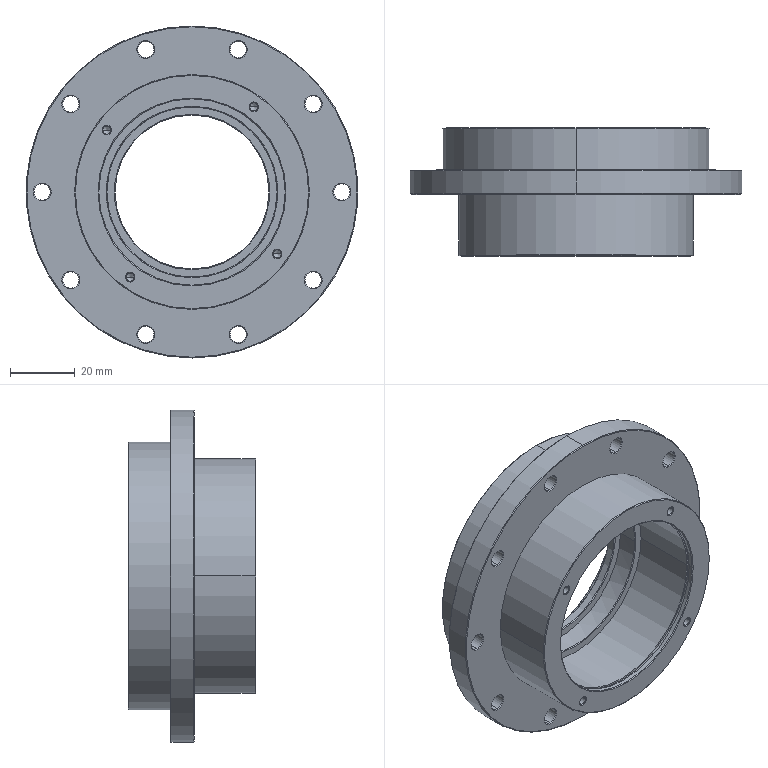Part | STEP file | 2026.6.15-Main Assembly图.sldasm-Part-90 | 1 solid | 129 faces | box 102.5 x 39.5 x 102.5 mm | volume 102953 mm3 | cone 74 | cylinder 46 | plane 9 | commonest cylinder face diameters 5 x20 2.5 x8 57.5 x4 47.5 x2 52.5 x2 58.5 x2